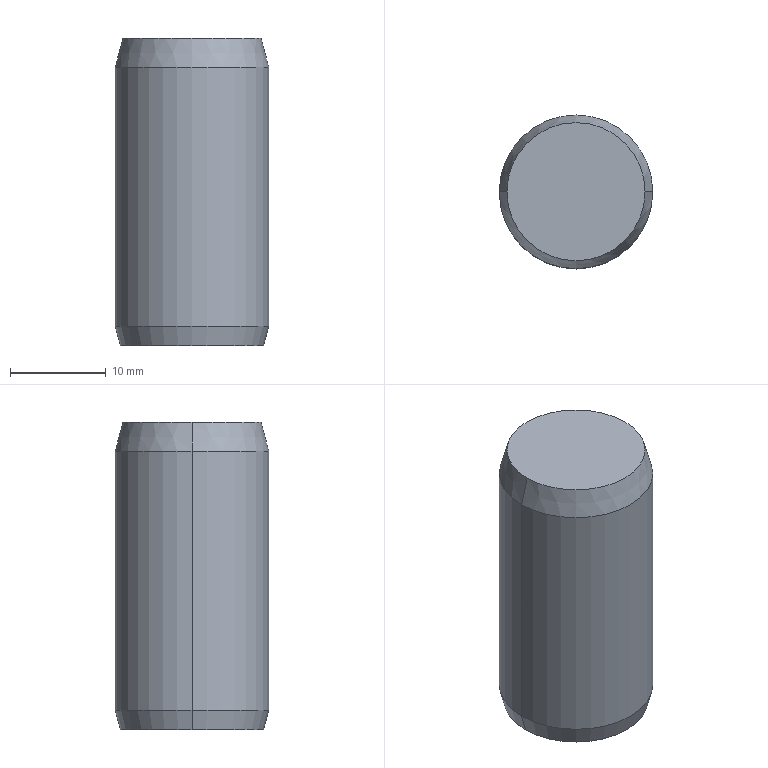Part | SolidWorks | features Chamfer 3, Cut 2, Extrusion 1, RevCut 1 | 1 solid | 16 faces | box 16 x 16 x 32 mm | volume 5349 mm3 | cone 8 | cylinder 6 | plane 2 | commonest cylinder face diameters 6.928 x2 8.4 x2 16 x2
STEP:
#1=CARTESIAN_POINT('',(3.464,0.,2.236));
#2=VERTEX_POINT('',#1);
#3=CARTESIAN_POINT('',(-3.464,0.,2.236));
#4=VERTEX_POINT('',#3);
#5=CARTESIAN_POINT('',(0.,0.,2.236));
#6=DIRECTION('',(0.,0.,-1.));
#7=DIRECTION('',(-1.,0.,0.));
#8=AXIS2_PLACEMENT_3D('',#5,#6,#7);
#9=CIRCLE('',#8,3.464);
#10=EDGE_CURVE('',#2,#4,#9,.T.);
#11=ORIENTED_EDGE('',*,*,#10,.F.);
#12=CARTESIAN_POINT('',(4.2,0.,1.5));
#13=VERTEX_POINT('',#12);
#14=CARTESIAN_POINT('',(4.2,0.,1.5));
#15=DIRECTION('',(0.7071,0.,-0.7071));
#16=VECTOR('',#15,1000.);
#17=LINE('',#14,#16);
#18=EDGE_CURVE('',#2,#13,#17,.T.);
#19=ORIENTED_EDGE('',*,*,#18,.T.);
#20=CARTESIAN_POINT('',(-4.2,0.,1.5));
#21=VERTEX_POINT('',#20);
#22=CARTESIAN_POINT('',(0.,0.,1.5));
#23=DIRECTION('',(0.,0.,-1.));
#24=DIRECTION('',(-1.,0.,0.));
#25=AXIS2_PLACEMENT_3D('',#22,#23,#24);
#26=CIRCLE('',#25,4.2);
#27=EDGE_CURVE('',#13,#21,#26,.T.);
#28=ORIENTED_EDGE('',*,*,#27,.T.);
#29=CARTESIAN_POINT('',(-4.2,0.,1.5));
#30=DIRECTION('',(-0.7071,0.,-0.7071));
#31=VECTOR('',#30,1000.);
#32=LINE('',#29,#31);
#33=EDGE_CURVE('',#4,#21,#32,.T.);
#34=ORIENTED_EDGE('',*,*,#33,.F.);
#35=EDGE_LOOP('',(#11,#19,#28,#34));
#36=FACE_OUTER_BOUND('',#35,.T.);
#37=CARTESIAN_POINT('',(0.,0.,1.5));
#38=DIRECTION('',(0.,0.,-1.));
#39=DIRECTION('',(-1.,0.,0.));
#40=AXIS2_PLACEMENT_3D('',#37,#38,#39);
#41=CONICAL_SURFACE('',#40,4.2,0.7854);
#42=ADVANCED_FACE('',(#36),#41,.F.);
#43=CARTESIAN_POINT('',(-3.464,0.,25.));
#44=VERTEX_POINT('',#43);
#45=CARTESIAN_POINT('',(3.464,0.,25.));
#46=VERTEX_POINT('',#45);
#47=CARTESIAN_POINT('',(0.,0.,25.));
#48=DIRECTION('',(0.,0.,1.));
#49=DIRECTION('',(1.,0.,0.));
#50=AXIS2_PLACEMENT_3D('',#47,#48,#49);
#51=CIRCLE('',#50,3.464);
#52=EDGE_CURVE('',#44,#46,#51,.T.);
#53=ORIENTED_EDGE('',*,*,#52,.T.);
#54=CARTESIAN_POINT('',(3.464,0.,25.));
#55=DIRECTION('',(0.,0.,-1.));
#56=VECTOR('',#55,1000.);
#57=LINE('',#54,#56);
#58=EDGE_CURVE('',#46,#2,#57,.T.);
#59=ORIENTED_EDGE('',*,*,#58,.T.);
#60=ORIENTED_EDGE('',*,*,#10,.T.);
#61=CARTESIAN_POINT('',(-3.464,0.,25.));
#62=DIRECTION('',(0.,0.,-1.));
#63=VECTOR('',#62,1000.);
#64=LINE('',#61,#63);
#65=EDGE_CURVE('',#44,#4,#64,.T.);
#66=ORIENTED_EDGE('',*,*,#65,.F.);
#67=EDGE_LOOP('',(#53,#59,#60,#66));
#68=FACE_OUTER_BOUND('',#67,.T.);
#69=CARTESIAN_POINT('',(0.,0.,25.));
#70=DIRECTION('',(0.,0.,-1.));
#71=DIRECTION('',(-1.,0.,0.));
#72=AXIS2_PLACEMENT_3D('',#69,#70,#71);
#73=CYLINDRICAL_SURFACE('',#72,3.464);
#74=ADVANCED_FACE('',(#68),#73,.F.);
#75=CARTESIAN_POINT('',(0.,0.,27.));
#76=VERTEX_POINT('',#75);
#77=CARTESIAN_POINT('',(-3.464,0.,25.));
#78=DIRECTION('',(-0.866,0.,-0.5));
#79=VECTOR('',#78,1000.);
#80=LINE('',#77,#79);
#81=EDGE_CURVE('',#76,#44,#80,.T.);
#82=ORIENTED_EDGE('',*,*,#81,.F.);
#83=CARTESIAN_POINT('',(3.464,0.,25.));
#84=DIRECTION('',(0.866,0.,-0.5));
#85=VECTOR('',#84,1000.);
#86=LINE('',#83,#85);
#87=EDGE_CURVE('',#76,#46,#86,.T.);
#88=ORIENTED_EDGE('',*,*,#87,.T.);
#89=ORIENTED_EDGE('',*,*,#52,.F.);
#90=EDGE_LOOP('',(#82,#88,#89));
#91=FACE_OUTER_BOUND('',#90,.T.);
#92=CARTESIAN_POINT('',(0.,0.,25.));
#93=DIRECTION('',(0.,0.,-1.));
#94=DIRECTION('',(-1.,0.,0.));
#95=AXIS2_PLACEMENT_3D('',#92,#93,#94);
#96=CONICAL_SURFACE('',#95,3.464,1.047);
#97=ADVANCED_FACE('',(#91),#96,.F.);
#98=ORIENTED_EDGE('',*,*,#27,.F.);
#99=CARTESIAN_POINT('',(4.2,0.,0.));
#100=VERTEX_POINT('',#99);
#101=CARTESIAN_POINT('',(4.2,0.,1.5));
#102=DIRECTION('',(0.,0.,-1.));
#103=VECTOR('',#102,1000.);
#104=LINE('',#101,#103);
#105=EDGE_CURVE('',#13,#100,#104,.T.);
#106=ORIENTED_EDGE('',*,*,#105,.T.);
#107=CARTESIAN_POINT('',(-4.2,0.,0.));
#108=VERTEX_POINT('',#107);
#109=CARTESIAN_POINT('',(0.,0.,0.));
#110=DIRECTION('',(0.,0.,-1.));
#111=DIRECTION('',(-1.,0.,0.));
#112=AXIS2_PLACEMENT_3D('',#109,#110,#111);
#113=CIRCLE('',#112,4.2);
#114=EDGE_CURVE('',#100,#108,#113,.T.);
#115=ORIENTED_EDGE('',*,*,#114,.T.);
#116=CARTESIAN_POINT('',(-4.2,0.,1.5));
#117=DIRECTION('',(0.,0.,-1.));
#118=VECTOR('',#117,1000.);
#119=LINE('',#116,#118);
#120=EDGE_CURVE('',#21,#108,#119,.T.);
#121=ORIENTED_EDGE('',*,*,#120,.F.);
#122=EDGE_LOOP('',(#98,#106,#115,#121));
#123=FACE_OUTER_BOUND('',#122,.T.);
#124=CARTESIAN_POINT('',(0.,0.,1.5));
#125=DIRECTION('',(0.,0.,-1.));
#126=DIRECTION('',(-1.,0.,0.));
#127=AXIS2_PLACEMENT_3D('',#124,#125,#126);
#128=CYLINDRICAL_SURFACE('',#127,4.2);
#129=ADVANCED_FACE('',(#123),#128,.F.);
#130=CARTESIAN_POINT('',(-7.464,0.,0.));
#131=VERTEX_POINT('',#130);
#132=CARTESIAN_POINT('',(7.464,0.,0.));
#133=VERTEX_POINT('',#132);
#134=CARTESIAN_POINT('',(0.,0.,0.));
#135=DIRECTION('',(0.,0.,-1.));
#136=DIRECTION('',(1.,0.,0.));
#137=AXIS2_PLACEMENT_3D('',#134,#135,#136);
#138=CIRCLE('',#137,7.464);
#139=EDGE_CURVE('',#131,#133,#138,.T.);
#140=ORIENTED_EDGE('',*,*,#139,.F.);
#141=CARTESIAN_POINT('',(-8.,0.,2.));
#142=VERTEX_POINT('',#141);
#143=CARTESIAN_POINT('',(-8.,0.,2.));
#144=DIRECTION('',(-0.2588,0.,0.9659));
#145=VECTOR('',#144,1000.);
#146=LINE('',#143,#145);
#147=EDGE_CURVE('',#131,#142,#146,.T.);
#148=ORIENTED_EDGE('',*,*,#147,.T.);
#149=CARTESIAN_POINT('',(8.,0.,2.));
#150=VERTEX_POINT('',#149);
#151=CARTESIAN_POINT('',(0.,0.,2.));
#152=DIRECTION('',(0.,0.,1.));
#153=DIRECTION('',(1.,0.,0.));
#154=AXIS2_PLACEMENT_3D('',#151,#152,#153);
#155=CIRCLE('',#154,8.);
#156=EDGE_CURVE('',#150,#142,#155,.T.);
#157=ORIENTED_EDGE('',*,*,#156,.F.);
#158=CARTESIAN_POINT('',(8.,0.,2.));
#159=DIRECTION('',(0.2588,0.,0.9659));
#160=VECTOR('',#159,1000.);
#161=LINE('',#158,#160);
#162=EDGE_CURVE('',#133,#150,#161,.T.);
#163=ORIENTED_EDGE('',*,*,#162,.F.);
#164=EDGE_LOOP('',(#140,#148,#157,#163));
#165=FACE_OUTER_BOUND('',#164,.T.);
#166=CARTESIAN_POINT('',(0.,0.,2.));
#167=DIRECTION('',(0.,0.,1.));
#168=DIRECTION('',(1.,0.,0.));
#169=AXIS2_PLACEMENT_3D('',#166,#167,#168);
#170=CONICAL_SURFACE('',#169,8.,0.2618);
#171=ADVANCED_FACE('',(#165),#170,.T.);
#172=CARTESIAN_POINT('',(7.196,0.,32.));
#173=VERTEX_POINT('',#172);
#174=CARTESIAN_POINT('',(-7.196,0.,32.));
#175=VERTEX_POINT('',#174);
#176=CARTESIAN_POINT('',(0.,0.,32.));
#177=DIRECTION('',(0.,0.,1.));
#178=DIRECTION('',(1.,0.,0.));
#179=AXIS2_PLACEMENT_3D('',#176,#177,#178);
#180=CIRCLE('',#179,7.196);
#181=EDGE_CURVE('',#173,#175,#180,.T.);
#182=ORIENTED_EDGE('',*,*,#181,.F.);
#183=CARTESIAN_POINT('',(8.,0.,29.));
#184=VERTEX_POINT('',#183);
#185=CARTESIAN_POINT('',(7.196,0.,32.));
#186=DIRECTION('',(0.2588,0.,-0.9659));
#187=VECTOR('',#186,1000.);
#188=LINE('',#185,#187);
#189=EDGE_CURVE('',#173,#184,#188,.T.);
#190=ORIENTED_EDGE('',*,*,#189,.T.);
#191=CARTESIAN_POINT('',(-8.,0.,29.));
#192=VERTEX_POINT('',#191);
#193=CARTESIAN_POINT('',(0.,0.,29.));
#194=DIRECTION('',(0.,0.,-1.));
#195=DIRECTION('',(1.,0.,0.));
#196=AXIS2_PLACEMENT_3D('',#193,#194,#195);
#197=CIRCLE('',#196,8.);
#198=EDGE_CURVE('',#192,#184,#197,.T.);
#199=ORIENTED_EDGE('',*,*,#198,.F.);
#200=CARTESIAN_POINT('',(-7.196,0.,32.));
#201=DIRECTION('',(-0.2588,0.,-0.9659));
#202=VECTOR('',#201,1000.);
#203=LINE('',#200,#202);
#204=EDGE_CURVE('',#175,#192,#203,.T.);
#205=ORIENTED_EDGE('',*,*,#204,.F.);
#206=EDGE_LOOP('',(#182,#190,#199,#205));
#207=FACE_OUTER_BOUND('',#206,.T.);
#208=CARTESIAN_POINT('',(0.,0.,32.));
#209=DIRECTION('',(0.,0.,-1.));
#210=DIRECTION('',(-1.,0.,0.));
#211=AXIS2_PLACEMENT_3D('',#208,#209,#210);
#212=CONICAL_SURFACE('',#211,7.196,0.2618);
#213=ADVANCED_FACE('',(#207),#212,.T.);
#214=ORIENTED_EDGE('',*,*,#198,.T.);
#215=CARTESIAN_POINT('',(8.,0.,32.));
#216=DIRECTION('',(0.,0.,-1.));
#217=VECTOR('',#216,1000.);
#218=LINE('',#215,#217);
#219=EDGE_CURVE('',#184,#150,#218,.T.);
#220=ORIENTED_EDGE('',*,*,#219,.T.);
#221=ORIENTED_EDGE('',*,*,#156,.T.);
#222=CARTESIAN_POINT('',(-8.,0.,32.));
#223=DIRECTION('',(0.,0.,-1.));
#224=VECTOR('',#223,1000.);
#225=LINE('',#222,#224);
#226=EDGE_CURVE('',#192,#142,#225,.T.);
#227=ORIENTED_EDGE('',*,*,#226,.F.);
#228=EDGE_LOOP('',(#214,#220,#221,#227));
#229=FACE_OUTER_BOUND('',#228,.T.);
#230=CARTESIAN_POINT('',(0.,0.,32.));
#231=DIRECTION('',(0.,0.,-1.));
#232=DIRECTION('',(-1.,0.,0.));
#233=AXIS2_PLACEMENT_3D('',#230,#231,#232);
#234=CYLINDRICAL_SURFACE('',#233,8.);
#235=ADVANCED_FACE('',(#229),#234,.T.);
#236=ORIENTED_EDGE('',*,*,#219,.F.);
#237=CARTESIAN_POINT('',(0.,0.,29.));
#238=DIRECTION('',(0.,0.,-1.));
#239=DIRECTION('',(1.,0.,0.));
#240=AXIS2_PLACEMENT_3D('',#237,#238,#239);
#241=CIRCLE('',#240,8.);
#242=EDGE_CURVE('',#184,#192,#241,.T.);
#243=ORIENTED_EDGE('',*,*,#242,.T.);
#244=ORIENTED_EDGE('',*,*,#226,.T.);
#245=CARTESIAN_POINT('',(0.,0.,2.));
#246=DIRECTION('',(0.,0.,1.));
#247=DIRECTION('',(1.,0.,0.));
#248=AXIS2_PLACEMENT_3D('',#245,#246,#247);
#249=CIRCLE('',#248,8.);
#250=EDGE_CURVE('',#142,#150,#249,.T.);
#251=ORIENTED_EDGE('',*,*,#250,.T.);
#252=EDGE_LOOP('',(#236,#243,#244,#251));
#253=FACE_OUTER_BOUND('',#252,.T.);
#254=CARTESIAN_POINT('',(0.,0.,32.));
#255=DIRECTION('',(0.,0.,-1.));
#256=DIRECTION('',(-1.,0.,0.));
#257=AXIS2_PLACEMENT_3D('',#254,#255,#256);
#258=CYLINDRICAL_SURFACE('',#257,8.);
#259=ADVANCED_FACE('',(#253),#258,.T.);
#260=CARTESIAN_POINT('',(0.,0.,32.));
#261=DIRECTION('',(0.,0.,1.));
#262=DIRECTION('',(1.,0.,0.));
#263=AXIS2_PLACEMENT_3D('',#260,#261,#262);
#264=CIRCLE('',#263,7.196);
#265=EDGE_CURVE('',#175,#173,#264,.T.);
#266=ORIENTED_EDGE('',*,*,#265,.T.);
#267=ORIENTED_EDGE('',*,*,#181,.T.);
#268=EDGE_LOOP('',(#266,#267));
#269=FACE_OUTER_BOUND('',#268,.T.);
#270=CARTESIAN_POINT('',(0.,0.,32.));
#271=DIRECTION('',(0.,0.,1.));
#272=DIRECTION('',(1.,0.,0.));
#273=AXIS2_PLACEMENT_3D('',#270,#271,#272);
#274=PLANE('',#273);
#275=ADVANCED_FACE('',(#269),#274,.T.);
#276=CARTESIAN_POINT('',(0.,0.,0.));
#277=DIRECTION('',(0.,0.,-1.));
#278=DIRECTION('',(-1.,0.,0.));
#279=AXIS2_PLACEMENT_3D('',#276,#277,#278);
#280=CIRCLE('',#279,4.2);
#281=EDGE_CURVE('',#108,#100,#280,.T.);
#282=ORIENTED_EDGE('',*,*,#281,.F.);
#283=ORIENTED_EDGE('',*,*,#114,.F.);
#284=EDGE_LOOP('',(#282,#283));
#285=FACE_BOUND('',#284,.T.);
#286=CARTESIAN_POINT('',(0.,0.,0.));
#287=DIRECTION('',(0.,0.,-1.));
#288=DIRECTION('',(1.,0.,0.));
#289=AXIS2_PLACEMENT_3D('',#286,#287,#288);
#290=CIRCLE('',#289,7.464);
#291=EDGE_CURVE('',#133,#131,#290,.T.);
#292=ORIENTED_EDGE('',*,*,#291,.T.);
#293=ORIENTED_EDGE('',*,*,#139,.T.);
#294=EDGE_LOOP('',(#292,#293));
#295=FACE_OUTER_BOUND('',#294,.T.);
#296=CARTESIAN_POINT('',(0.,0.,0.));
#297=DIRECTION('',(0.,0.,1.));
#298=DIRECTION('',(1.,0.,0.));
#299=AXIS2_PLACEMENT_3D('',#296,#297,#298);
#300=PLANE('',#299);
#301=ADVANCED_FACE('',(#285,#295),#300,.F.);
#302=ORIENTED_EDGE('',*,*,#189,.F.);
#303=ORIENTED_EDGE('',*,*,#265,.F.);
#304=ORIENTED_EDGE('',*,*,#204,.T.);
#305=ORIENTED_EDGE('',*,*,#242,.F.);
#306=EDGE_LOOP('',(#302,#303,#304,#305));
#307=FACE_OUTER_BOUND('',#306,.T.);
#308=CARTESIAN_POINT('',(0.,0.,32.));
#309=DIRECTION('',(0.,0.,-1.));
#310=DIRECTION('',(-1.,0.,0.));
#311=AXIS2_PLACEMENT_3D('',#308,#309,#310);
#312=CONICAL_SURFACE('',#311,7.196,0.2618);
#313=ADVANCED_FACE('',(#307),#312,.T.);
#314=ORIENTED_EDGE('',*,*,#147,.F.);
#315=ORIENTED_EDGE('',*,*,#291,.F.);
#316=ORIENTED_EDGE('',*,*,#162,.T.);
#317=ORIENTED_EDGE('',*,*,#250,.F.);
#318=EDGE_LOOP('',(#314,#315,#316,#317));
#319=FACE_OUTER_BOUND('',#318,.T.);
#320=CARTESIAN_POINT('',(0.,0.,2.));
#321=DIRECTION('',(0.,0.,1.));
#322=DIRECTION('',(1.,0.,0.));
#323=AXIS2_PLACEMENT_3D('',#320,#321,#322);
#324=CONICAL_SURFACE('',#323,8.,0.2618);
#325=ADVANCED_FACE('',(#319),#324,.T.);
#326=ORIENTED_EDGE('',*,*,#105,.F.);
#327=CARTESIAN_POINT('',(0.,0.,1.5));
#328=DIRECTION('',(0.,0.,-1.));
#329=DIRECTION('',(-1.,0.,0.));
#330=AXIS2_PLACEMENT_3D('',#327,#328,#329);
#331=CIRCLE('',#330,4.2);
#332=EDGE_CURVE('',#21,#13,#331,.T.);
#333=ORIENTED_EDGE('',*,*,#332,.F.);
#334=ORIENTED_EDGE('',*,*,#120,.T.);
#335=ORIENTED_EDGE('',*,*,#281,.T.);
#336=EDGE_LOOP('',(#326,#333,#334,#335));
#337=FACE_OUTER_BOUND('',#336,.T.);
#338=CARTESIAN_POINT('',(0.,0.,1.5));
#339=DIRECTION('',(0.,0.,-1.));
#340=DIRECTION('',(-1.,0.,0.));
#341=AXIS2_PLACEMENT_3D('',#338,#339,#340);
#342=CYLINDRICAL_SURFACE('',#341,4.2);
#343=ADVANCED_FACE('',(#337),#342,.F.);
#344=ORIENTED_EDGE('',*,*,#87,.F.);
#345=ORIENTED_EDGE('',*,*,#81,.T.);
#346=CARTESIAN_POINT('',(0.,0.,25.));
#347=DIRECTION('',(0.,0.,1.));
#348=DIRECTION('',(1.,0.,0.));
#349=AXIS2_PLACEMENT_3D('',#346,#347,#348);
#350=CIRCLE('',#349,3.464);
#351=EDGE_CURVE('',#46,#44,#350,.T.);
#352=ORIENTED_EDGE('',*,*,#351,.F.);
#353=EDGE_LOOP('',(#344,#345,#352));
#354=FACE_OUTER_BOUND('',#353,.T.);
#355=CARTESIAN_POINT('',(0.,0.,25.));
#356=DIRECTION('',(0.,0.,-1.));
#357=DIRECTION('',(-1.,0.,0.));
#358=AXIS2_PLACEMENT_3D('',#355,#356,#357);
#359=CONICAL_SURFACE('',#358,3.464,1.047);
#360=ADVANCED_FACE('',(#354),#359,.F.);
#361=ORIENTED_EDGE('',*,*,#58,.F.);
#362=ORIENTED_EDGE('',*,*,#351,.T.);
#363=ORIENTED_EDGE('',*,*,#65,.T.);
#364=CARTESIAN_POINT('',(0.,0.,2.236));
#365=DIRECTION('',(0.,0.,-1.));
#366=DIRECTION('',(-1.,0.,0.));
#367=AXIS2_PLACEMENT_3D('',#364,#365,#366);
#368=CIRCLE('',#367,3.464);
#369=EDGE_CURVE('',#4,#2,#368,.T.);
#370=ORIENTED_EDGE('',*,*,#369,.T.);
#371=EDGE_LOOP('',(#361,#362,#363,#370));
#372=FACE_OUTER_BOUND('',#371,.T.);
#373=CARTESIAN_POINT('',(0.,0.,25.));
#374=DIRECTION('',(0.,0.,-1.));
#375=DIRECTION('',(-1.,0.,0.));
#376=AXIS2_PLACEMENT_3D('',#373,#374,#375);
#377=CYLINDRICAL_SURFACE('',#376,3.464);
#378=ADVANCED_FACE('',(#372),#377,.F.);
#379=ORIENTED_EDGE('',*,*,#18,.F.);
#380=ORIENTED_EDGE('',*,*,#369,.F.);
#381=ORIENTED_EDGE('',*,*,#33,.T.);
#382=ORIENTED_EDGE('',*,*,#332,.T.);
#383=EDGE_LOOP('',(#379,#380,#381,#382));
#384=FACE_OUTER_BOUND('',#383,.T.);
#385=CARTESIAN_POINT('',(0.,0.,1.5));
#386=DIRECTION('',(0.,0.,-1.));
#387=DIRECTION('',(-1.,0.,0.));
#388=AXIS2_PLACEMENT_3D('',#385,#386,#387);
#389=CONICAL_SURFACE('',#388,4.2,0.7854);
#390=ADVANCED_FACE('',(#384),#389,.F.);
#391=CLOSED_SHELL('',(#42,#74,#97,#129,#171,#213,#235,#259,#275,#301,#313,#325,#343,#360,#378,#390));
#392=MANIFOLD_SOLID_BREP('',#391);
#393=CARTESIAN_POINT('',(0.,0.,0.));
#394=DIRECTION('',(0.,0.,1.));
#395=DIRECTION('',(1.,0.,0.));
#396=AXIS2_PLACEMENT_3D('',#393,#394,#395);
#397=(LENGTH_UNIT()NAMED_UNIT(*)SI_UNIT(.MILLI.,.METRE.));
#398=UNCERTAINTY_MEASURE_WITH_UNIT(LENGTH_MEASURE(0.00001),#397,'','');
#399=(NAMED_UNIT(*)PLANE_ANGLE_UNIT()SI_UNIT($,.RADIAN.));
#400=(NAMED_UNIT(*)SI_UNIT($,.STERADIAN.)SOLID_ANGLE_UNIT());
#401=(GEOMETRIC_REPRESENTATION_CONTEXT(3)GLOBAL_UNCERTAINTY_ASSIGNED_CONTEXT((#398))GLOBAL_UNIT_ASSIGNED_CONTEXT((#397,#399,#400))REPRESENTATION_CONTEXT('',''));
#402=ADVANCED_BREP_SHAPE_REPRESENTATION('',(#392,#396),#401);